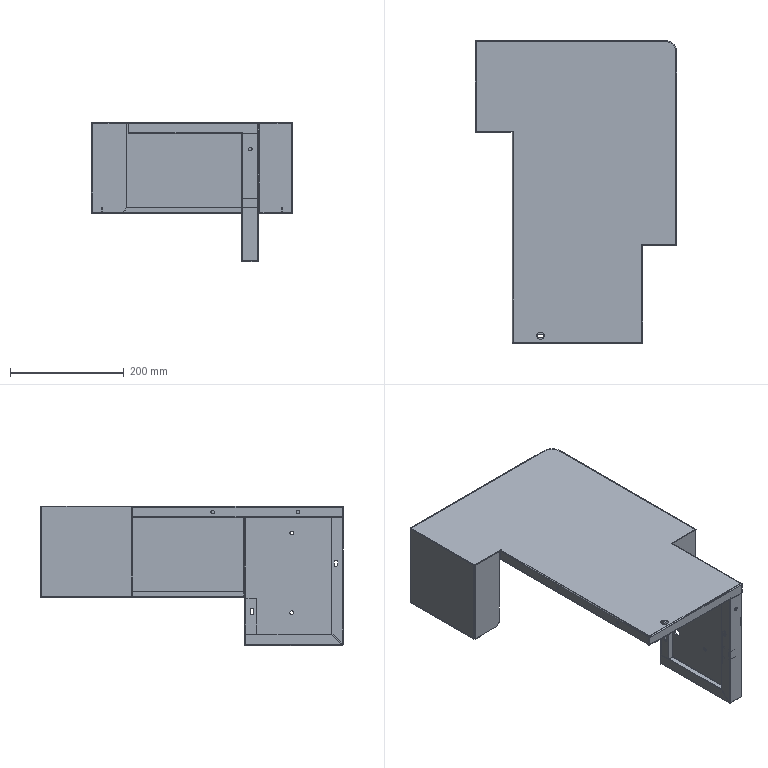Part | SolidWorks | 4 solids | 308 faces | box 355 x 533 x 245 mm | volume 625684 mm3 | plane 221 | cylinder 81 | spline 6 | commonest cylinder face diameters 4 x21 1 x20 6.4 x14 6 x7 13 x6 3 x3